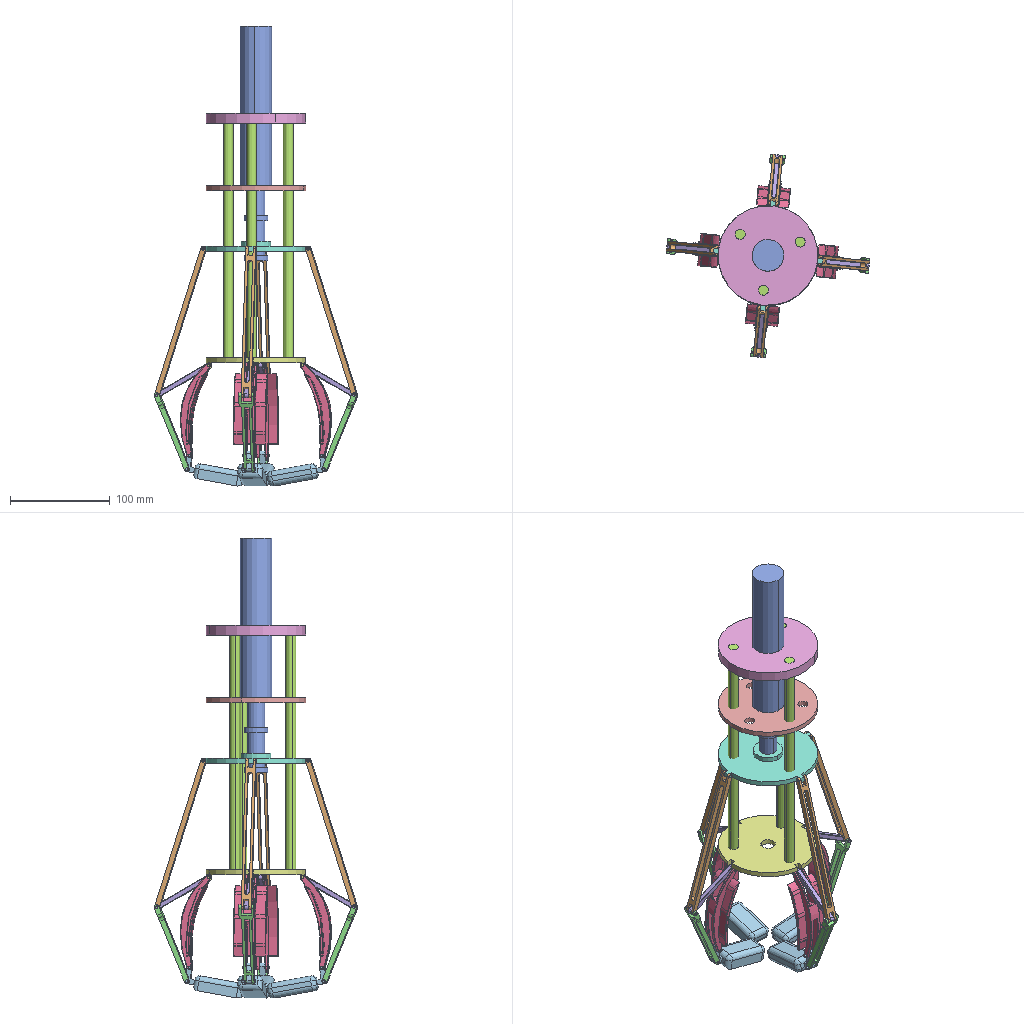Assembly | SolidWorks | 11 different items | 28 placed | box 204 x 204 x 461 mm
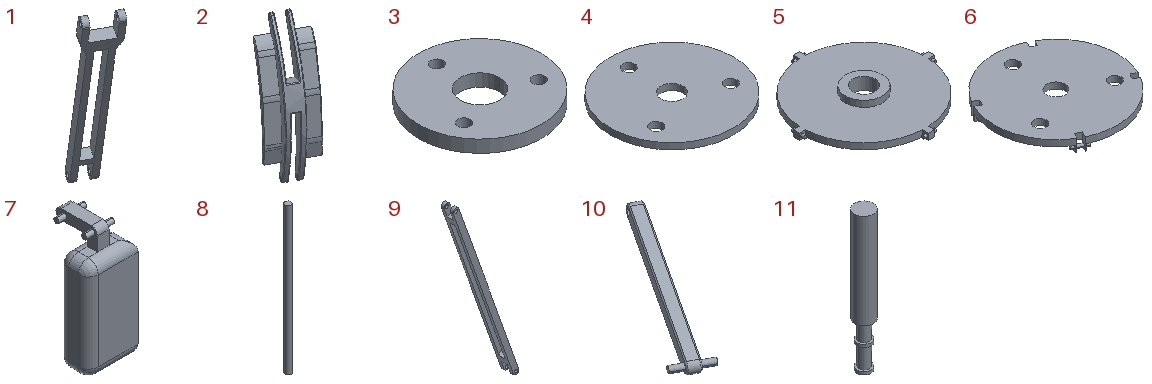Parts list (item | quantity | size | volume | features):
1 | x4 | 24.253 x 30.565 x 81.628 mm | 2325 mm3 | features ICE 7, HoleWzd 4, Extrusion 1
2 | x4 | 37.754 x 33.673 x 94.864 mm | 10570 mm3 | features Chamfer 5, HoleWzd 4, RefSurface 2, ThickenCut 2, BaseBody 1, Fillet 1
3 | x1 | 100 x 100 x 10 mm | 68141 mm3 | features ICE 2, CirPattern 1, Extrusion 1
4 | x1 | 100 x 100 x 5 mm | 36819 mm3 | features ICE 2, CirPattern 1, Extrusion 1
5 | x1 | 110 x 110 x 10 mm | 40860 mm3 | features ICE 4, CirPattern 1, Extrusion 1
6 | x1 | - | - | features ICE 5, Revolution 4, CirPattern 2, HoleWzd 2, RefSurface 2
7 | x4 | 25 x 25.958 x 60 mm | 18052 mm3 | features ICE 3, Fillet 2, Extrusion 1
8 | x3 | 10 x 10 x 250 mm | 19635 mm3 | features Extrusion 1
9 | x4 | 57.658 x 11.753 x 149.475 mm | 4168 mm3 | features ICE 4, HoleWzd 2, Extrusion 1
10 | x4 | 37.545 x 58.428 x 22.236 mm | 1589 mm3 | features Revolution 2, Chamfer 1, Extrusion 1, HoleWzd 1
11 | x1 | 32 x 32 x 235 mm | 149708 mm3 | features ICE 4, LPattern 1
Mates (type | each side: item.copy, entity, surface, feature):
Concentric | assembly face | 4.1 face cylinder Cut-Extrude2
Concentric | 4.1 face cylinder Cut-Extrude2 | assembly face
Concentric | assembly face | assembly face | 30 times
Coincident | assembly face | assembly face | 22 times
Parallel | 4.1 face cylinder CirPattern1 | assembly face
Concentric | assembly face | 4.1 face cylinder Cut-Extrude1
Concentric | 4.1 face cylinder Cut-Extrude1 | assembly face
Concentric | assembly face | 11.1 face cylinder Boss-Extrude2
Coincident | assembly face | 11.1 face
Concentric | assembly face | 8.1 face cylinder Boss-Extrude1
Coincident | assembly face | 8.1 face plane Boss-Extrude1 | 2 times
Concentric | assembly face | 8.2 face cylinder Boss-Extrude1
Coincident | assembly face | 8.2 face plane Boss-Extrude1 | 2 times
Concentric | assembly face | 8.3 face cylinder Boss-Extrude1 | 2 times
Coincident | assembly face | 8.3 face plane Boss-Extrude1 | 2 times
Concentric | 8.3 face cylinder Boss-Extrude1 | 3.1 face cylinder CirPattern1
Concentric | 11.1 face cylinder Boss-Extrude1 | 3.1 face cylinder Cut-Extrude2
Coincident | 8.3 face plane Boss-Extrude1 | 3.1 face plane Boss-Extrude1
Concentric | 8.2 face cylinder Boss-Extrude1 | 3.1 face cylinder CirPattern1
Concentric | 11.1 face cylinder Boss-Extrude2 | 5.1 face cylinder Cut-Extrude1
Concentric | assembly face | 5.1 face cylinder CirPattern3
Concentric | 11.1 face cylinder Boss-Extrude2 | 6.1 face cylinder Ø15.0 (15) Diameter Hole1
Concentric | 4.1 face cylinder Cut-Extrude2 | 11.1 face cylinder Boss-Extrude2
Coincident | 4.1 edge | 11.1 face plane Boss-Extrude1
Concentric | 8.1 face cylinder Boss-Extrude1 | 3.1 face cylinder Cut-Extrude1
Coincident | 8.1 face plane Boss-Extrude1 | 3.1 face plane Boss-Extrude1
Concentric | 8.1 face cylinder Boss-Extrude1 | 6.1 face cylinder Cut-Extrude4
Concentric | 5.1 face cylinder Boss-Extrude4 | 9.1 face cylinder Ø2.5 (2.5) Diameter Hole1
Coincident | 5.1 face plane Boss-Extrude3 | 9.1 face plane Cut-Extrude1
Coincident | 8.1 face plane Boss-Extrude1 | 6.1 face plane Revolve1
Coincident | 8.2 face plane Boss-Extrude1 | 6.1 face plane Revolve1
Concentric | 5.1 face cylinder CirPattern3 | assembly face | 2 times
Coincident | 5.1 face plane CirPattern3 | assembly face | 2 times
Concentric | 6.1 face cylinder Revolve4 | 10.1 face cylinder Ø2.5 (2.5) Diameter Hole1
Concentric | 9.1 face cylinder Ø2.5 (2.5) Diameter Hole1 | 10.1 face cylinder Revolve1
Coincident | 6.1 face plane Cut-Extrude1 | 10.1 face plane Boss-Extrude1
Concentric | 6.1 face | assembly face | 2 times
Coincident | 6.1 face | assembly face | 2 times
Concentric | 10.1 face cylinder Revolve1 | 1.1 face cylinder Ø2.5 (2.5) Diameter Hole3
Coincident | 9.1 face plane Boss-Extrude1 | 1.1 face plane Cut-Extrude3
Concentric | 6.1 face cylinder Revolve2 | 2.1 face cylinder Ø2.5 (2.5) Diameter Hole1
Coincident | 6.1 face plane Boss-Extrude5 | 2.1 face plane Cut-Thicken2
Concentric | 1.1 face cylinder Ø2.5 (2.5) Diameter Hole2 | assembly face
Concentric | 1.1 face cylinder Ø2.5 (2.5) Diameter Hole1 | 7.1 face cylinder Boss-Extrude4
Concentric | 2.1 face cylinder Ø2.5 (2.5) Diameter Hole2 | 7.1 face cylinder Boss-Extrude4
Coincident | 1.1 face plane Cut-Extrude1 | 7.1 face plane Boss-Extrude2